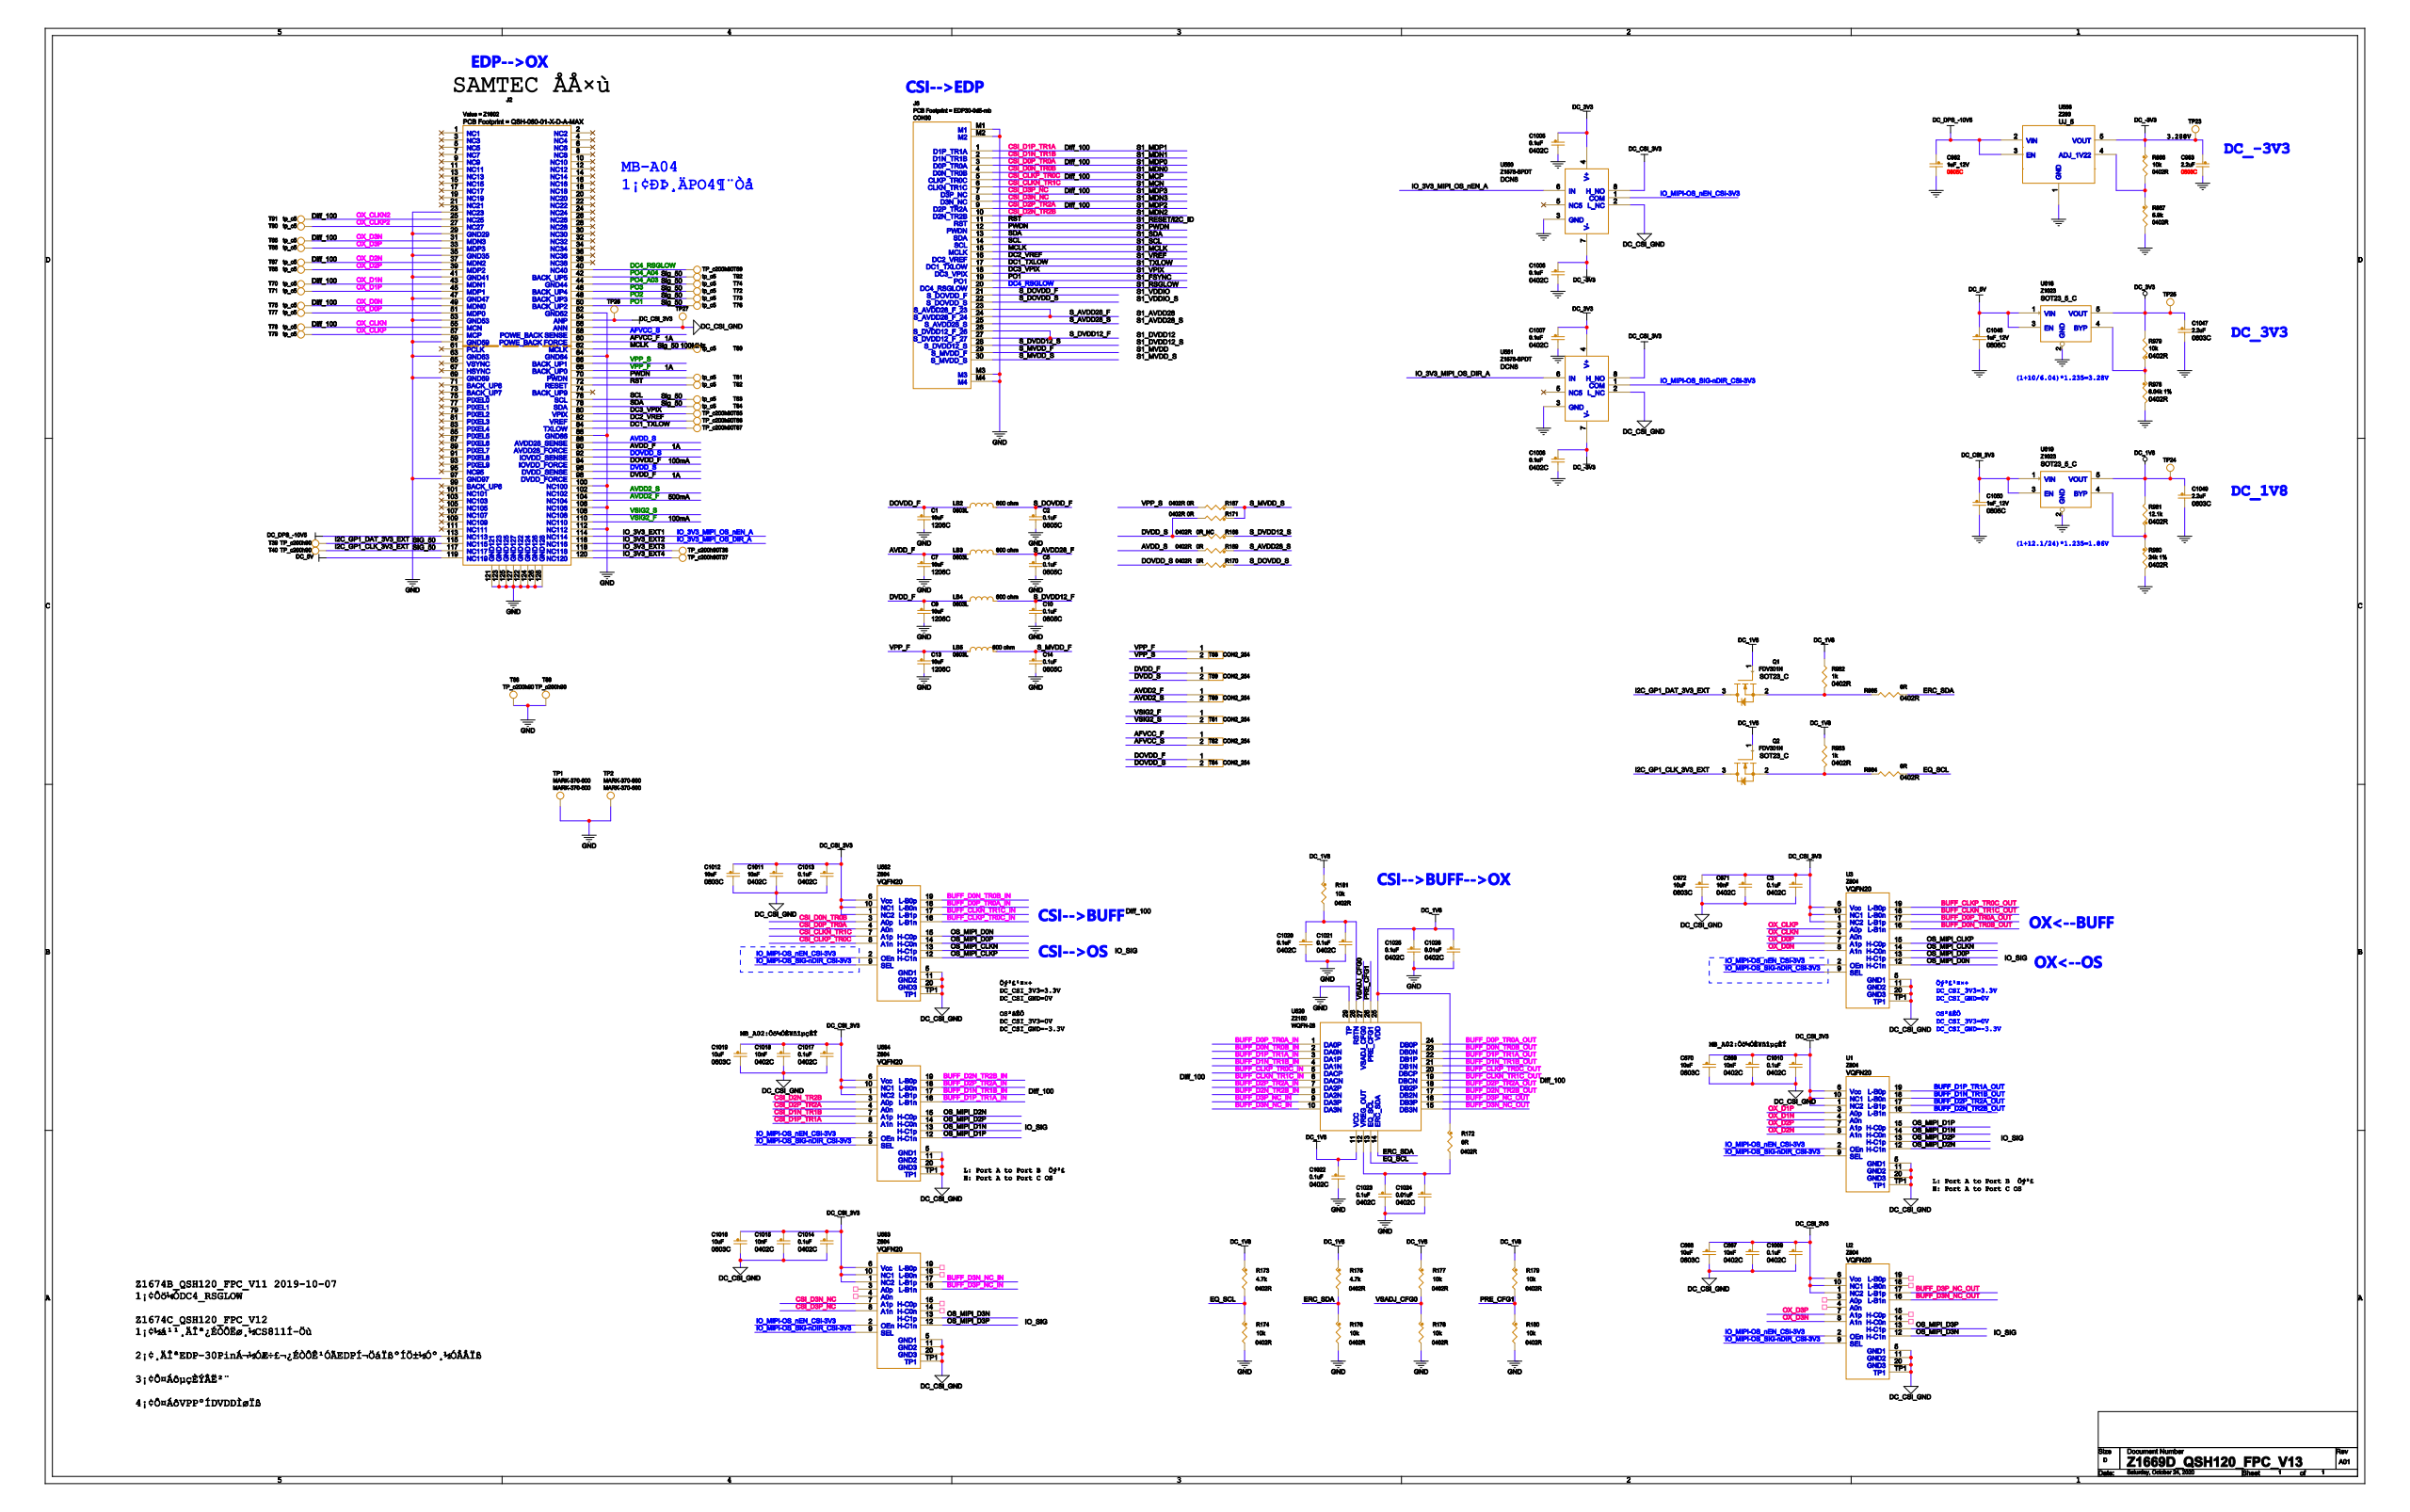Circuit board | Cadence Allegro | 133 parts | 115 nets
Bill of materials:
SYM_NAME,COMP_DEVICE_TYPE,COMP_VALUE,COMP_TOL,COMP_CLASS,REFDES
1206C,CAP_NP_C_1206C_DISCRETE_10UF_,10uF,,DISCRETE,C1
0805C,CAP_NP_C_0805C_DISCRETE_0.1UF_,0.1uF,,DISCRETE,C2
0402C,CAP_NP_C_0402C_DISCRETE_0.1UF_,0.1uF,,DISCRETE,C3
0805C,CAP_NP_C_0805C_DISCRETE_0.1UF_,0.1uF,,DISCRETE,C5
1206C,CAP_NP_C_1206C_DISCRETE_10UF_,10uF,,DISCRETE,C7
1206C,CAP_NP_C_1206C_DISCRETE_10UF_,10uF,,DISCRETE,C9
0805C,CAP_NP_C_0805C_DISCRETE_0.1UF_,0.1uF,,DISCRETE,C10
1206C,CAP_NP_C_1206C_DISCRETE_10UF_,10uF,,DISCRETE,C13
0805C,CAP_NP_C_0805C_DISCRETE_0.1UF_,0.1uF,,DISCRETE,C14
0402C,CAP_NP_C_0402C_DISCRETE_10NF,10nF,,DISCRETE,C667
0603C,CAP_NP_C_0603C_DISCRETE_10UF,10uF,,DISCRETE,C668
0402C,CAP_NP_C_0402C_DISCRETE_10NF,10nF,,DISCRETE,C669
0603C,CAP_NP_C_0603C_DISCRETE_10UF,10uF,,DISCRETE,C670
0402C,CAP_NP_C_0402C_DISCRETE_10NF,10nF,,DISCRETE,C671
0603C,CAP_NP_C_0603C_DISCRETE_10UF,10uF,,DISCRETE,C672
0805C,CAP_NP_C_0805C_DISCRETE_1UF_12V,1uF_12V,,DISCRETE,C962
0603C,CAP_NP_C_0603C_DISCRETE_2.2UF,2.2uF,,DISCRETE,C963
0402C,CAP_NP_C_0402C_DISCRETE_0.1UF,0.1uF,,DISCRETE,C1005
0402C,CAP_NP_C_0402C_DISCRETE_0.1UF,0.1uF,,DISCRETE,C1006
0402C,CAP_NP_C_0402C_DISCRETE_0.1UF,0.1uF,,DISCRETE,C1007
0402C,CAP_NP_C_0402C_DISCRETE_0.1UF,0.1uF,,DISCRETE,C1008
0402C,CAP_NP_C_0402C_DISCRETE_0.1UF,0.1uF,,DISCRETE,C1009
0402C,CAP_NP_C_0402C_DISCRETE_0.1UF,0.1uF,,DISCRETE,C1010
0402C,CAP_NP_C_0402C_DISCRETE_10NF,10nF,,DISCRETE,C1011
0603C,CAP_NP_C_0603C_DISCRETE_10UF,10uF,,DISCRETE,C1012
0402C,CAP_NP_C_0402C_DISCRETE_0.1UF_,0.1uF,,DISCRETE,C1013
0402C,CAP_NP_C_0402C_DISCRETE_0.1UF,0.1uF,,DISCRETE,C1014
0402C,CAP_NP_C_0402C_DISCRETE_10NF,10nF,,DISCRETE,C1015
0603C,CAP_NP_C_0603C_DISCRETE_10UF,10uF,,DISCRETE,C1016
0402C,CAP_NP_C_0402C_DISCRETE_0.1UF,0.1uF,,DISCRETE,C1017
0402C,CAP_NP_C_0402C_DISCRETE_10NF,10nF,,DISCRETE,C1018
0603C,CAP_NP_C_0603C_DISCRETE_10UF,10uF,,DISCRETE,C1019
0402C,CAP_NP_C_0402C_DISCRETE_0.1UF,0.1uF,,DISCRETE,C1020
0402C,CAP_NP_C_0402C_DISCRETE_0.1UF,0.1uF,,DISCRETE,C1021
0402C,CAP_NP_C_0402C_DISCRETE_0.1UF,0.1uF,,DISCRETE,C1022
0402C,CAP_NP_C_0402C_DISCRETE_0.1UF,0.1uF,,DISCRETE,C1023
0402C,CAP_NP_C_0402C_DISCRETE_0.01UF,0.01uF,,DISCRETE,C1024
0402C,CAP_NP_C_0402C_DISCRETE_0.1UF,0.1uF,,DISCRETE,C1025
0402C,CAP_NP_C_0402C_DISCRETE_0.01UF,0.01uF,,DISCRETE,C1026
0603C,CAP_NP_C_0603C_DISCRETE_2.2UF,2.2uF,,DISCRETE,C1047
0805C,CAP_NP_C_0805C_DISCRETE_1UF_12V,1uF_12V,,DISCRETE,C1048
0603C,CAP_NP_C_0603C_DISCRETE_2.2UF,2.2uF,,DISCRETE,C1049
0805C,CAP_NP_C_0805C_DISCRETE_1UF_12V,1uF_12V,,DISCRETE,C1050
QSH-060-01-X-D-A-MAX,QTH-060-01-L-D-A_QSH-060-01-X-D,Z1602,,IC,J2
EDP30-0D5-MB,COM30P_EDP_D05_1_EDP30-0D5-MB_C,CON30,,IC,J6
0603L,L_0603L_600 OHM_,600 ohm,,IC,LB2
0603L,L_0603L_600 OHM_,600 ohm,,IC,LB3
0603L,L_0603L_600 OHM_,600 ohm,,IC,LB4
0603L,L_0603L_600 OHM_,600 ohm,,IC,LB5
SOT23_C,MOSFET_N_GSD_C1_SOT23_C_FDV301N,FDV301N,,IC,Q1
SOT23_C,MOSFET_N_GSD_C1_SOT23_C_FDV301N,FDV301N,,IC,Q2
0402R,RES_C1_0402R_DISCRETE_0R,0R,,DISCRETE,R167
0402R,RES_C1_0402R_DISCRETE_0R_NC,0R_NC,,DISCRETE,R168
0402R,RES_C1_0402R_DISCRETE_0R,0R,,DISCRETE,R169
0402R,RES_C1_0402R_DISCRETE_0R,0R,,DISCRETE,R170
0402R,RES_C1_0402R_DISCRETE_0R,0R,,DISCRETE,R171
0402R,RES_C1_0402R_DISCRETE_0R,0R,,DISCRETE,R172
0402R,RES_C1_0402R_DISCRETE_4.7K,4.7k,,DISCRETE,R173
0402R,RES_C1_0402R_DISCRETE_10K,10k,,DISCRETE,R174
0402R,RES_C1_0402R_DISCRETE_4.7K,4.7k,,DISCRETE,R175
0402R,RES_C1_0402R_DISCRETE_10K,10k,,DISCRETE,R176
0402R,RES_C1_0402R_DISCRETE_10K,10k,,DISCRETE,R177
0402R,RES_C1_0402R_DISCRETE_10K,10k,,DISCRETE,R178
0402R,RES_C1_0402R_DISCRETE_10K,10k,,DISCRETE,R179
0402R,RES_C1_0402R_DISCRETE_10K,10k,,DISCRETE,R180
0402R,RES_C1_0402R_DISCRETE_10K,10k,,DISCRETE,R181
0402R,RES_C1_0402R_DISCRETE_10K,10k,,DISCRETE,R866
0402R,RES_C1_0402R_DISCRETE_5.9K,5.9k,,DISCRETE,R867
0402R,RES_C1_0402R_DISCRETE_6.04K 1%,6.04k 1%,,DISCRETE,R978
0402R,RES_C1_0402R_DISCRETE_10K,10k,,DISCRETE,R979
0402R,RES_C1_0402R_DISCRETE_24K 1%,24k 1%,,DISCRETE,R980
0402R,RES_C1_0402R_DISCRETE_12.1K,12.1k,,DISCRETE,R981
0402R,R_0402R_1K_,1k,,IC,R982
0402R,R_0402R_1K_,1k,,IC,R983
0402R,R_0402R_0R_,0R,,IC,R984
0402R,R_0402R_0R_,0R,,IC,R985
TP_C200H90,TP_TP_C200H90_T POINT R,T POINT R,,IC,T36
TP_C200H90,TP_TP_C200H90_T POINT R,T POINT R,,IC,T37
TP_C200H90,TP_TP_C200H90_T POINT R,T POINT R,,IC,T39
TP_C200H90,TP_TP_C200H90_T POINT R,T POINT R,,IC,T40
CON2_254,CON2_0_CON2_254_CON2,CON2,,IC,T58
CON2_254,CON2_0_CON2_254_CON2,CON2,,IC,T59
CON2_254,CON2_0_CON2_254_CON2,CON2,,IC,T60
CON2_254,CON2_0_CON2_254_CON2,CON2,,IC,T61
CON2_254,CON2_0_CON2_254_CON2,CON2,,IC,T62
CON2_254,CON2_0_CON2_254_CON2,CON2,,IC,T64
TP_C5,TP_TP_C5_T POINT R,T POINT R,,IC,T65
TP_C5,TP_TP_C5_T POINT R,T POINT R,,IC,T66
TP_C5,TP_TP_C5_T POINT R,T POINT R,,IC,T67
TP_C5,TP_TP_C5_T POINT R,T POINT R,,IC,T68
TP_C200H90,TP_TP_C200H90_T POINT R,T POINT R,,IC,T69
TP_C5,TP_TP_C5_T POINT R,T POINT R,,IC,T70
TP_C5,TP_TP_C5_T POINT R,T POINT R,,IC,T71
TP_C5,TP_TP_C5_T POINT R,T POINT R,,IC,T72
TP_C5,TP_TP_C5_T POINT R,T POINT R,,IC,T73
TP_C5,TP_TP_C5_T POINT R,T POINT R,,IC,T74
TP_C5,TP_TP_C5_T POINT R,T POINT R,,IC,T75
TP_C5,TP_TP_C5_T POINT R,T POINT R,,IC,T76
TP_C5,TP_TP_C5_T POINT R,T POINT R,,IC,T77
TP_C5,TP_TP_C5_T POINT R,T POINT R,,IC,T78
TP_C5,TP_TP_C5_T POINT R,T POINT R,,IC,T79
TP_C5,TP_TP_C5_T POINT R,T POINT R,,IC,T80
TP_C5,TP_TP_C5_T POINT R,T POINT R,,IC,T81
TP_C5,TP_TP_C5_T POINT R,T POINT R,,IC,T82
TP_C5,TP_TP_C5_T POINT R,T POINT R,,IC,T83
TP_C5,TP_TP_C5_T POINT R,T POINT R,,IC,T84
TP_C200H90,TP_TP_C200H90_T POINT R,T POINT R,,IC,T85
TP_C200H90,TP_TP_C200H90_T POINT R,T POINT R,,IC,T86
TP_C200H90,TP_TP_C200H90_T POINT R,T POINT R,,IC,T87
TP_C200H90,TP_TP_C200H90_T POINT R,T POINT R,,IC,T88
TP_C200H90,TP_TP_C200H90_T POINT R,T POINT R,,IC,T89
TP_C5,TP_TP_C5_T POINT R,T POINT R,,IC,T90
TP_C5,TP_TP_C5_T POINT R,T POINT R,,IC,T91
TP_C5,TP_TP_C5_T POINT R,T POINT R,,IC,T92
MARK-370-600,TP_MARK-370-600_MARK-370-600,MARK-370-600,,IC,TP1
MARK-370-600,TP_MARK-370-600_MARK-370-600,MARK-370-600,,IC,TP2
TP_C5,T POINT R_TP_C5_T POINT R,T POINT R,,IC,TP23
TP_C5,T POINT R_TP_C5_T POINT R,T POINT R,,IC,TP24
TP_C5,T POINT R_TP_C5_T POINT R,T POINT R,,IC,TP25
TP_C5,T POINT R_TP_C5_T POINT R,T POINT R,,IC,TP26
TP_C5,T POINT R_TP_C5_T POINT R,T POINT R,,IC,TP27
VQFN20,Z804_0_VQFN20_Z804,Z804,,IC,U1
VQFN20,Z804_0_VQFN20_Z804,Z804,,IC,U2
VQFN20,Z804_0_VQFN20_Z804,Z804,,IC,U3
UJ_5,Z1572_UJ_5_Z293,Z293,,IC,U566
DCN8,20-1121-SPDT_7_DCN8_Z1578-SPDT,Z1578-SPDT,,IC,U580
DCN8,20-1121-SPDT_7_DCN8_Z1578-SPDT,Z1578-SPDT,,IC,U581
VQFN20,Z804_0_VQFN20_Z804,Z804,,IC,U582
VQFN20,Z804_0_VQFN20_Z804,Z804,,IC,U583
VQFN20,Z804_0_VQFN20_Z804,Z804,,IC,U584
SOT23_5_C,SPX5205_SOT23_5_C_Z1023,Z1023,,IC,U618
SOT23_5_C,SPX5205_SOT23_5_C_Z1023,Z1023,,IC,U619
WQFN-28,SN75DPHY_0_WQFN-28_Z2150,Z2150,,IC,U620
Netlist (net: part-pin ...):
N1438955: Q2-2 R983-2 R984-1
EQ_SCL: R173-2 R174-1 R984-2 U620-13
N1438879: Q1-2 R982-2 R985-1
ERC_SDA: R175-2 R176-1 R985-2 U620-14
DC_CSI_GND: C3-2 C667-2 C668-2 C669-2 C670-2 C671-2 C672-2 C1009-2 C1010-2 C1011-2 C1012-2 C1013-2 C1014-2 C1015-2 C1016-2 C1017-2 C1018-2 C1019-2 J2-56 TP27-1 U1-5 U1-11 U1-20 U1-TP1 U2-5 U2-11 U2-20 U2-TP1 U3-5 U3-11 U3-20 U3-TP1 U580-2 U581-2 U582-5 U582-11 U582-20 U582-TP1 U583-5 U583-11 U583-20 U583-TP1 U584-5 U584-11 U584-20 U584-TP1
DC_CSI_3V3: C3-1 C667-1 C668-1 C669-1 C670-1 C671-1 C672-1 C1009-1 C1010-1 C1011-1 C1012-1 C1013-1 C1014-1 C1015-1 C1016-1 C1017-1 C1018-1 C1019-1 C1050-1 J2-54 TP26-1 U1-1 U1-6 U1-10 U2-1 U2-6 U2-10 U3-1 U3-6 U3-10 U580-8 U581-8 U582-1 U582-6 U582-10 U583-1 U583-6 U583-10 U584-1 U584-6 U584-10 U619-1 U619-3
AVDD_F: C7-1 J2-90 LB3-1
AVDD_S: J2-88 R169-2
VPP_F: C13-1 J2-68 LB5-1 T58-1
VPP_S: J2-66 R167-2 T58-2
PO1: J2-50 J6-19 T76-1
PO2: J2-48 T73-1
PO3: J2-46 T72-1
PO4_A04: J2-42 T92-1
DVDD_F: C9-1 J2-98 LB4-1 T59-1
DVDD_S: J2-96 R168-2 R171-2 T59-2
GND: C1-2 C2-2 C5-2 C7-2 C9-2 C10-2 C13-2 C14-2 C962-2 C963-2 C1005-2 C1006-2 C1007-2 C1008-2 C1020-2 C1021-2 C1022-2 C1023-2 C1024-2 C1025-2 C1026-2 C1047-2 C1048-2 C1049-2 C1050-2 J2-23 J2-29 J2-35 J2-41 J2-47 J2-52 J2-53 J2-59 J2-63 J2-64 J2-69 J2-86 J2-97 J2-100 J2-106 J2-112 J2-121 J2-122 J2-123 J2-124 J2-125 J2-126 J2-127 J2-128 J6-M1 J6-M2 J6-M3 J6-M4 R174-2 R176-2 R178-2 R180-2 R867-2 R978-2 R980-2 T88-1 T89-1 TP1-1 TP2-1 U566-1 U580-3 U581-3 U618-2 U619-2 U620-29
PO4_A03: J2-44 T74-1
DOVDD_F: C1-1 J2-94 LB2-1 T64-1
DOVDD_S: J2-92 R170-2 T64-2
MCLK: J2-62 J6-15 T80-1
OX_CLKN: J2-55 T78-1 U3-4
OX_CLKP: J2-57 T79-1 U3-3
OX_D0N: J2-49 T75-1 U3-8
OX_D1N: J2-43 T70-1 U1-4
OX_D2N: J2-37 T67-1 U1-8
OX_D3N: J2-31 T65-1 U2-8
OX_D0P: J2-51 T77-1 U3-7
OX_D1P: J2-45 T71-1 U1-3
OX_D2P: J2-39 T68-1 U1-7
OX_D3P: J2-33 T66-1 U2-7
AVDD2_S: J2-102 T60-2
AVDD2_F: J2-104 T60-1
VSIG2_S: J2-108 T61-2
VSIG2_F: J2-110 T61-1
DC_DPS_-10V5: C962-1 J2-113 U566-2 U566-3
IO_3V3_EXT1: J2-114 U580-6
I2C_GP1_DAT_3V3_EXT: J2-115 Q1-3 T39-1
IO_3V3_EXT2: J2-116 U581-6
I2C_GP1_CLK_3V3_EXT: J2-117 Q2-3 T40-1
IO_3V3_EXT3: J2-118 T36-1
DC_5V: C1048-1 J2-119 U618-1 U618-3
IO_3V3_EXT4: J2-120 T37-1
OX_CLKN2: J2-25 T91-1
OX_CLKP2: J2-27 T90-1
DC4_RSGLOW: J2-40 J6-20 T69-1
AFVCC_F: J2-60 T62-1
AFVCC_S: J2-58 T62-2
PWDN: J2-70 J6-12 T81-1
RST: J2-72 J6-11 T82-1
SCL: J2-76 J6-14 T83-1
SDA: J2-78 J6-13 T84-1
DC1_TXLOW: J2-84 J6-17 T87-1
DC3_VPIX: J2-80 J6-18 T85-1
DC2_VREF: J2-82 J6-16 T86-1
BUFF_D0N_TR0B_IN: U582-19 U620-2
BUFF_D0P_TR0A_IN: U582-18 U620-1
BUFF_D1N_TR1B_IN: U584-17 U620-4
BUFF_D1P_TR1A_IN: U584-16 U620-3
BUFF_D2N_TR2B_IN: U584-19 U620-8
BUFF_D2P_TR2A_IN: U584-18 U620-7
BUFF_D3N_NC_IN: U583-17 U620-10
BUFF_D3P_NC_IN: U583-16 U620-9
BUFF_CLKN_TR1C_IN: U582-17 U620-6
BUFF_CLKP_TR0C_IN: U582-16 U620-5
BUFF_D0N_TR0B_OUT: U3-16 U620-23
BUFF_D0P_TR0A_OUT: U3-17 U620-24
BUFF_D1N_TR1B_OUT: U1-18 U620-21
BUFF_D1P_TR1A_OUT: U1-19 U620-22
BUFF_D2N_TR2B_OUT: U1-16 U620-17
BUFF_D2P_TR2A_OUT: U1-17 U620-18
BUFF_D3N_NC_OUT: U2-16 U620-15
BUFF_D3P_NC_OUT: U2-17 U620-16
BUFF_CLKN_TR1C_OUT: U3-18 U620-19
BUFF_CLKP_TR0C_OUT: U3-19 U620-20
PRE_CFG1: R179-2 R180-1 U620-26
N1432020: C1020-1 C1021-1 R181-2 U620-28
DC_1V8: C1022-1 C1025-1 C1026-1 C1049-1 Q1-1 Q2-1 R172-1 R173-1 R175-1 R177-1 R179-1 R181-1 R981-2 R982-1 R983-1 TP24-1 U619-5 U620-11 U620-25
N1434782: C1023-1 C1024-1 R172-2 U620-12
VSADJ_CFG0: R177-2 R178-1 U620-27
S_DVDD12_F: C10-1 J6-26 J6-27 LB4-2
S_MVDD_F: C14-1 J6-29 LB5-2
S_DOVDD_F: C2-1 J6-21 LB2-2
S_AVDD28_F: C5-1 J6-23 J6-24 LB3-2
DC_3V3: C1005-1 C1007-1 C1047-1 R979-2 TP25-1 U580-4 U581-4 U618-5
DC_-3V3: C963-1 C1006-1 C1008-1 R866-1 TP23-1 U566-5 U580-7 U581-7
CSI_D1P_TR1A: J6-1 U584-8
CSI_D2N_TR2B: J6-10 U584-3
CSI_D1N_TR1B: J6-2 U584-7
S_DOVDD_S: J6-22 R170-1
S_AVDD28_S: J6-25 R169-1
S_DVDD12_S: J6-28 R168-1
CSI_D0P_TR0A: J6-3 U582-4
S_MVDD_S: J6-30 R167-1 R171-1
CSI_D0N_TR0B: J6-4 U582-3
CSI_CLKP_TR0C: J6-5 U582-8
CSI_CLKN_TR1C: J6-6 U582-7
CSI_D3P_NC: J6-7 U583-8
CSI_D3N_NC: J6-8 U583-7
CSI_D2P_TR2A: J6-9 U584-4
N1445301: R866-2 R867-1 U566-4
N1446179: R978-1 R979-1 U618-4
N1447499: R980-1 R981-1 U619-4
OS_MIPI_D1N: U1-14 U584-13
OS_MIPI_D1P: U1-15 U584-12
OS_MIPI_D2N: U1-12 U584-15
OS_MIPI_D2P: U1-13 U584-14
IO_MIPI-OS_NEN_CSI-3V3: U1-2 U2-2 U3-2 U580-1 U582-2 U583-2 U584-2
IO_MIPI-OS_SIG-NDIR_CSI-3V3: U1-9 U2-9 U3-9 U581-1 U582-9 U583-9 U584-9
OS_MIPI_D3N: U2-12 U583-13
OS_MIPI_D3P: U2-13 U583-12
OS_MIPI_CLKN: U3-14 U582-13
OS_MIPI_CLKP: U3-15 U582-12
OS_MIPI_D0N: U3-12 U582-15
OS_MIPI_D0P: U3-13 U582-14